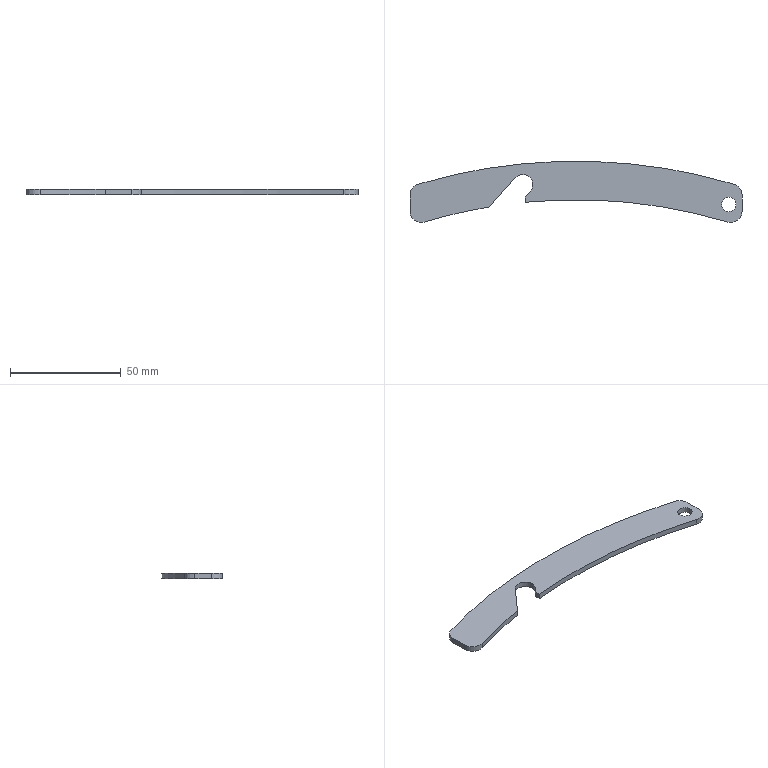Part | SolidWorks | features Fillet 1, FlatPattern 1, ICE 1, SMBaseFlange 1, SheetMetal 1 | 1 solid | 18 faces | box 150 x 27.697 x 2.5 mm | volume 6095 mm3 | cylinder 11 | plane 7 | commonest cylinder face diameters 10 x4 6.5 x2 9 x2 477.484 x2 500 x1
STEP:
#1=CARTESIAN_POINT('',(65.75,-8.,-2.5));
#2=VERTEX_POINT('',#1);
#3=CARTESIAN_POINT('',(72.25,-8.,-2.5));
#4=VERTEX_POINT('',#3);
#5=CARTESIAN_POINT('',(69.,-8.,-2.5));
#6=DIRECTION('',(0.,0.,1.));
#7=DIRECTION('',(1.,0.,0.));
#8=AXIS2_PLACEMENT_3D('',#5,#6,#7);
#9=CIRCLE('',#8,3.25);
#10=EDGE_CURVE('',#2,#4,#9,.T.);
#11=ORIENTED_EDGE('',*,*,#10,.F.);
#12=CARTESIAN_POINT('',(65.75,-8.,0.));
#13=VERTEX_POINT('',#12);
#14=CARTESIAN_POINT('',(65.75,-8.,-2.5));
#15=DIRECTION('',(0.,0.,1.));
#16=VECTOR('',#15,1000.);
#17=LINE('',#14,#16);
#18=EDGE_CURVE('',#2,#13,#17,.T.);
#19=ORIENTED_EDGE('',*,*,#18,.T.);
#20=CARTESIAN_POINT('',(72.25,-8.,0.));
#21=VERTEX_POINT('',#20);
#22=CARTESIAN_POINT('',(69.,-8.,0.));
#23=DIRECTION('',(0.,0.,1.));
#24=DIRECTION('',(1.,0.,0.));
#25=AXIS2_PLACEMENT_3D('',#22,#23,#24);
#26=CIRCLE('',#25,3.25);
#27=EDGE_CURVE('',#13,#21,#26,.T.);
#28=ORIENTED_EDGE('',*,*,#27,.T.);
#29=CARTESIAN_POINT('',(72.25,-8.,-2.5));
#30=DIRECTION('',(0.,0.,1.));
#31=VECTOR('',#30,1000.);
#32=LINE('',#29,#31);
#33=EDGE_CURVE('',#4,#21,#32,.T.);
#34=ORIENTED_EDGE('',*,*,#33,.F.);
#35=EDGE_LOOP('',(#11,#19,#28,#34));
#36=FACE_OUTER_BOUND('',#35,.T.);
#37=CARTESIAN_POINT('',(69.,-8.,-2.5));
#38=DIRECTION('',(0.,0.,1.));
#39=DIRECTION('',(1.,0.,0.));
#40=AXIS2_PLACEMENT_3D('',#37,#38,#39);
#41=CYLINDRICAL_SURFACE('',#40,3.25);
#42=ADVANCED_FACE('',(#36),#41,.F.);
#43=CARTESIAN_POINT('',(-27.362,4.,-2.5));
#44=VERTEX_POINT('',#43);
#45=CARTESIAN_POINT('',(-19.508,1.,-2.5));
#46=VERTEX_POINT('',#45);
#47=CARTESIAN_POINT('',(-24.008,1.,-2.5));
#48=DIRECTION('',(0.,0.,-1.));
#49=DIRECTION('',(-1.,0.,0.));
#50=AXIS2_PLACEMENT_3D('',#47,#48,#49);
#51=CIRCLE('',#50,4.5);
#52=EDGE_CURVE('',#44,#46,#51,.T.);
#53=ORIENTED_EDGE('',*,*,#52,.T.);
#54=CARTESIAN_POINT('',(-19.508,1.,0.));
#55=VERTEX_POINT('',#54);
#56=CARTESIAN_POINT('',(-19.508,1.,-2.5));
#57=DIRECTION('',(0.,0.,1.));
#58=VECTOR('',#57,1000.);
#59=LINE('',#56,#58);
#60=EDGE_CURVE('',#46,#55,#59,.T.);
#61=ORIENTED_EDGE('',*,*,#60,.T.);
#62=CARTESIAN_POINT('',(-27.362,4.,0.));
#63=VERTEX_POINT('',#62);
#64=CARTESIAN_POINT('',(-24.008,1.,0.));
#65=DIRECTION('',(0.,0.,-1.));
#66=DIRECTION('',(-1.,0.,0.));
#67=AXIS2_PLACEMENT_3D('',#64,#65,#66);
#68=CIRCLE('',#67,4.5);
#69=EDGE_CURVE('',#63,#55,#68,.T.);
#70=ORIENTED_EDGE('',*,*,#69,.F.);
#71=CARTESIAN_POINT('',(-27.362,4.,-2.5));
#72=DIRECTION('',(0.,0.,1.));
#73=VECTOR('',#72,1000.);
#74=LINE('',#71,#73);
#75=EDGE_CURVE('',#44,#63,#74,.T.);
#76=ORIENTED_EDGE('',*,*,#75,.F.);
#77=EDGE_LOOP('',(#53,#61,#70,#76));
#78=FACE_OUTER_BOUND('',#77,.T.);
#79=CARTESIAN_POINT('',(-24.008,1.,-2.5));
#80=DIRECTION('',(0.,0.,1.));
#81=DIRECTION('',(1.,0.,0.));
#82=AXIS2_PLACEMENT_3D('',#79,#80,#81);
#83=CYLINDRICAL_SURFACE('',#82,4.5);
#84=ADVANCED_FACE('',(#78),#83,.F.);
#85=CARTESIAN_POINT('',(-23.008,-7.025,0.));
#86=VERTEX_POINT('',#85);
#87=CARTESIAN_POINT('',(68.564,-15.971,0.));
#88=VERTEX_POINT('',#87);
#89=CARTESIAN_POINT('',(0.,-244.656,0.));
#90=DIRECTION('',(0.,0.,-1.));
#91=DIRECTION('',(-1.,0.,0.));
#92=AXIS2_PLACEMENT_3D('',#89,#90,#91);
#93=CIRCLE('',#92,238.742);
#94=EDGE_CURVE('',#86,#88,#93,.T.);
#95=ORIENTED_EDGE('',*,*,#94,.F.);
#96=CARTESIAN_POINT('',(-23.008,-7.025,-2.5));
#97=VERTEX_POINT('',#96);
#98=CARTESIAN_POINT('',(-23.008,-7.025,-2.5));
#99=DIRECTION('',(0.,0.,1.));
#100=VECTOR('',#99,1000.);
#101=LINE('',#98,#100);
#102=EDGE_CURVE('',#97,#86,#101,.T.);
#103=ORIENTED_EDGE('',*,*,#102,.F.);
#104=CARTESIAN_POINT('',(68.564,-15.971,-2.5));
#105=VERTEX_POINT('',#104);
#106=CARTESIAN_POINT('',(0.,-244.656,-2.5));
#107=DIRECTION('',(0.,0.,-1.));
#108=DIRECTION('',(-1.,0.,0.));
#109=AXIS2_PLACEMENT_3D('',#106,#107,#108);
#110=CIRCLE('',#109,238.742);
#111=EDGE_CURVE('',#97,#105,#110,.T.);
#112=ORIENTED_EDGE('',*,*,#111,.T.);
#113=CARTESIAN_POINT('',(68.564,-15.971,-2.5));
#114=DIRECTION('',(0.,0.,1.));
#115=VECTOR('',#114,1000.);
#116=LINE('',#113,#115);
#117=EDGE_CURVE('',#105,#88,#116,.T.);
#118=ORIENTED_EDGE('',*,*,#117,.T.);
#119=EDGE_LOOP('',(#95,#103,#112,#118));
#120=FACE_OUTER_BOUND('',#119,.T.);
#121=CARTESIAN_POINT('',(0.,-244.656,-2.5));
#122=DIRECTION('',(0.,0.,1.));
#123=DIRECTION('',(1.,0.,0.));
#124=AXIS2_PLACEMENT_3D('',#121,#122,#123);
#125=CYLINDRICAL_SURFACE('',#124,238.742);
#126=ADVANCED_FACE('',(#120),#125,.F.);
#127=CARTESIAN_POINT('',(-20.654,-2.,-2.5));
#128=VERTEX_POINT('',#127);
#129=CARTESIAN_POINT('',(-23.008,-4.632,-2.5));
#130=VERTEX_POINT('',#129);
#131=CARTESIAN_POINT('',(-25.363,-7.265,-2.5));
#132=DIRECTION('',(-0.6667,-0.7454,0.));
#133=VECTOR('',#132,1000.);
#134=LINE('',#131,#133);
#135=EDGE_CURVE('',#128,#130,#134,.T.);
#136=ORIENTED_EDGE('',*,*,#135,.T.);
#137=CARTESIAN_POINT('',(-23.008,-4.632,0.));
#138=VERTEX_POINT('',#137);
#139=CARTESIAN_POINT('',(-23.008,-4.632,-2.5));
#140=DIRECTION('',(0.,0.,1.));
#141=VECTOR('',#140,1000.);
#142=LINE('',#139,#141);
#143=EDGE_CURVE('',#130,#138,#142,.T.);
#144=ORIENTED_EDGE('',*,*,#143,.T.);
#145=CARTESIAN_POINT('',(-20.654,-2.,0.));
#146=VERTEX_POINT('',#145);
#147=CARTESIAN_POINT('',(-25.363,-7.265,0.));
#148=DIRECTION('',(-0.6667,-0.7454,0.));
#149=VECTOR('',#148,1000.);
#150=LINE('',#147,#149);
#151=EDGE_CURVE('',#146,#138,#150,.T.);
#152=ORIENTED_EDGE('',*,*,#151,.F.);
#153=CARTESIAN_POINT('',(-20.654,-2.,-2.5));
#154=DIRECTION('',(0.,0.,1.));
#155=VECTOR('',#154,1000.);
#156=LINE('',#153,#155);
#157=EDGE_CURVE('',#128,#146,#156,.T.);
#158=ORIENTED_EDGE('',*,*,#157,.F.);
#159=EDGE_LOOP('',(#136,#144,#152,#158));
#160=FACE_OUTER_BOUND('',#159,.T.);
#161=CARTESIAN_POINT('',(-25.363,-7.265,-2.5));
#162=DIRECTION('',(-0.7454,0.6667,0.));
#163=DIRECTION('',(-0.6667,-0.7454,0.));
#164=AXIS2_PLACEMENT_3D('',#161,#162,#163);
#165=PLANE('',#164);
#166=ADVANCED_FACE('',(#160),#165,.T.);
#167=CARTESIAN_POINT('',(69.,-8.,-2.5));
#168=DIRECTION('',(0.,0.,1.));
#169=DIRECTION('',(1.,0.,0.));
#170=AXIS2_PLACEMENT_3D('',#167,#168,#169);
#171=CIRCLE('',#170,3.25);
#172=EDGE_CURVE('',#4,#2,#171,.T.);
#173=ORIENTED_EDGE('',*,*,#172,.T.);
#174=ORIENTED_EDGE('',*,*,#10,.T.);
#175=EDGE_LOOP('',(#173,#174));
#176=FACE_BOUND('',#175,.T.);
#177=ORIENTED_EDGE('',*,*,#111,.F.);
#178=CARTESIAN_POINT('',(-23.008,-238.485,-2.5));
#179=DIRECTION('',(0.,-1.,0.));
#180=VECTOR('',#179,1000.);
#181=LINE('',#178,#180);
#182=EDGE_CURVE('',#130,#97,#181,.T.);
#183=ORIENTED_EDGE('',*,*,#182,.F.);
#184=ORIENTED_EDGE('',*,*,#135,.F.);
#185=CARTESIAN_POINT('',(-24.008,1.,-2.5));
#186=DIRECTION('',(0.,0.,-1.));
#187=DIRECTION('',(-1.,0.,0.));
#188=AXIS2_PLACEMENT_3D('',#185,#186,#187);
#189=CIRCLE('',#188,4.5);
#190=EDGE_CURVE('',#46,#128,#189,.T.);
#191=ORIENTED_EDGE('',*,*,#190,.F.);
#192=ORIENTED_EDGE('',*,*,#52,.F.);
#193=CARTESIAN_POINT('',(-39.114,-9.139,-2.5));
#194=VERTEX_POINT('',#193);
#195=CARTESIAN_POINT('',(-27.362,4.,-2.5));
#196=DIRECTION('',(0.6667,0.7454,0.));
#197=VECTOR('',#196,1000.);
#198=LINE('',#195,#197);
#199=EDGE_CURVE('',#194,#44,#198,.T.);
#200=ORIENTED_EDGE('',*,*,#199,.F.);
#201=CARTESIAN_POINT('',(-68.564,-15.971,-2.5));
#202=VERTEX_POINT('',#201);
#203=CARTESIAN_POINT('',(0.,-244.656,-2.5));
#204=DIRECTION('',(0.,0.,-1.));
#205=DIRECTION('',(-1.,0.,0.));
#206=AXIS2_PLACEMENT_3D('',#203,#204,#205);
#207=CIRCLE('',#206,238.742);
#208=EDGE_CURVE('',#202,#194,#207,.T.);
#209=ORIENTED_EDGE('',*,*,#208,.F.);
#210=CARTESIAN_POINT('',(-75.,-11.181,-2.5));
#211=VERTEX_POINT('',#210);
#212=CARTESIAN_POINT('',(-70.,-11.181,-2.5));
#213=DIRECTION('',(0.,0.,-1.));
#214=DIRECTION('',(-1.,0.,0.));
#215=AXIS2_PLACEMENT_3D('',#212,#213,#214);
#216=CIRCLE('',#215,5.);
#217=EDGE_CURVE('',#202,#211,#216,.T.);
#218=ORIENTED_EDGE('',*,*,#217,.T.);
#219=CARTESIAN_POINT('',(-75.,-3.698,-2.5));
#220=VERTEX_POINT('',#219);
#221=CARTESIAN_POINT('',(-75.,0.,-2.5));
#222=DIRECTION('',(0.,-1.,0.));
#223=VECTOR('',#222,1000.);
#224=LINE('',#221,#223);
#225=EDGE_CURVE('',#220,#211,#224,.T.);
#226=ORIENTED_EDGE('',*,*,#225,.F.);
#227=CARTESIAN_POINT('',(-71.429,1.094,-2.5));
#228=VERTEX_POINT('',#227);
#229=CARTESIAN_POINT('',(-70.,-3.698,-2.5));
#230=DIRECTION('',(0.,0.,-1.));
#231=DIRECTION('',(-1.,0.,0.));
#232=AXIS2_PLACEMENT_3D('',#229,#230,#231);
#233=CIRCLE('',#232,5.);
#234=EDGE_CURVE('',#220,#228,#233,.T.);
#235=ORIENTED_EDGE('',*,*,#234,.T.);
#236=CARTESIAN_POINT('',(71.429,1.094,-2.5));
#237=VERTEX_POINT('',#236);
#238=CARTESIAN_POINT('',(0.,-238.485,-2.5));
#239=DIRECTION('',(0.,0.,1.));
#240=DIRECTION('',(-1.,0.,0.));
#241=AXIS2_PLACEMENT_3D('',#238,#239,#240);
#242=CIRCLE('',#241,250.);
#243=EDGE_CURVE('',#237,#228,#242,.T.);
#244=ORIENTED_EDGE('',*,*,#243,.F.);
#245=CARTESIAN_POINT('',(75.,-3.698,-2.5));
#246=VERTEX_POINT('',#245);
#247=CARTESIAN_POINT('',(70.,-3.698,-2.5));
#248=DIRECTION('',(0.,0.,-1.));
#249=DIRECTION('',(-1.,0.,0.));
#250=AXIS2_PLACEMENT_3D('',#247,#248,#249);
#251=CIRCLE('',#250,5.);
#252=EDGE_CURVE('',#237,#246,#251,.T.);
#253=ORIENTED_EDGE('',*,*,#252,.T.);
#254=CARTESIAN_POINT('',(75.,-11.181,-2.5));
#255=VERTEX_POINT('',#254);
#256=CARTESIAN_POINT('',(75.,0.,-2.5));
#257=DIRECTION('',(0.,1.,0.));
#258=VECTOR('',#257,1000.);
#259=LINE('',#256,#258);
#260=EDGE_CURVE('',#255,#246,#259,.T.);
#261=ORIENTED_EDGE('',*,*,#260,.F.);
#262=CARTESIAN_POINT('',(70.,-11.181,-2.5));
#263=DIRECTION('',(0.,0.,-1.));
#264=DIRECTION('',(-1.,0.,0.));
#265=AXIS2_PLACEMENT_3D('',#262,#263,#264);
#266=CIRCLE('',#265,5.);
#267=EDGE_CURVE('',#255,#105,#266,.T.);
#268=ORIENTED_EDGE('',*,*,#267,.T.);
#269=EDGE_LOOP('',(#177,#183,#184,#191,#192,#200,#209,#218,#226,#235,#244,#253,#261,#268));
#270=FACE_OUTER_BOUND('',#269,.T.);
#271=CARTESIAN_POINT('',(0.,-238.485,-2.5));
#272=DIRECTION('',(0.,0.,-1.));
#273=DIRECTION('',(-1.,0.,0.));
#274=AXIS2_PLACEMENT_3D('',#271,#272,#273);
#275=PLANE('',#274);
#276=ADVANCED_FACE('',(#176,#270),#275,.T.);
#277=CARTESIAN_POINT('',(69.,-8.,0.));
#278=DIRECTION('',(0.,0.,1.));
#279=DIRECTION('',(1.,0.,0.));
#280=AXIS2_PLACEMENT_3D('',#277,#278,#279);
#281=CIRCLE('',#280,3.25);
#282=EDGE_CURVE('',#21,#13,#281,.T.);
#283=ORIENTED_EDGE('',*,*,#282,.F.);
#284=ORIENTED_EDGE('',*,*,#27,.F.);
#285=EDGE_LOOP('',(#283,#284));
#286=FACE_BOUND('',#285,.T.);
#287=CARTESIAN_POINT('',(-23.008,-238.485,0.));
#288=DIRECTION('',(0.,-1.,0.));
#289=VECTOR('',#288,1000.);
#290=LINE('',#287,#289);
#291=EDGE_CURVE('',#138,#86,#290,.T.);
#292=ORIENTED_EDGE('',*,*,#291,.T.);
#293=ORIENTED_EDGE('',*,*,#94,.T.);
#294=CARTESIAN_POINT('',(75.,-11.181,0.));
#295=VERTEX_POINT('',#294);
#296=CARTESIAN_POINT('',(70.,-11.181,0.));
#297=DIRECTION('',(0.,0.,1.));
#298=DIRECTION('',(-1.,0.,0.));
#299=AXIS2_PLACEMENT_3D('',#296,#297,#298);
#300=CIRCLE('',#299,5.);
#301=EDGE_CURVE('',#88,#295,#300,.T.);
#302=ORIENTED_EDGE('',*,*,#301,.T.);
#303=CARTESIAN_POINT('',(75.,-3.698,0.));
#304=VERTEX_POINT('',#303);
#305=CARTESIAN_POINT('',(75.,0.,0.));
#306=DIRECTION('',(0.,1.,0.));
#307=VECTOR('',#306,1000.);
#308=LINE('',#305,#307);
#309=EDGE_CURVE('',#295,#304,#308,.T.);
#310=ORIENTED_EDGE('',*,*,#309,.T.);
#311=CARTESIAN_POINT('',(71.429,1.094,0.));
#312=VERTEX_POINT('',#311);
#313=CARTESIAN_POINT('',(70.,-3.698,0.));
#314=DIRECTION('',(0.,0.,1.));
#315=DIRECTION('',(-1.,0.,0.));
#316=AXIS2_PLACEMENT_3D('',#313,#314,#315);
#317=CIRCLE('',#316,5.);
#318=EDGE_CURVE('',#304,#312,#317,.T.);
#319=ORIENTED_EDGE('',*,*,#318,.T.);
#320=CARTESIAN_POINT('',(-71.429,1.094,0.));
#321=VERTEX_POINT('',#320);
#322=CARTESIAN_POINT('',(0.,-238.485,0.));
#323=DIRECTION('',(0.,0.,1.));
#324=DIRECTION('',(-1.,0.,0.));
#325=AXIS2_PLACEMENT_3D('',#322,#323,#324);
#326=CIRCLE('',#325,250.);
#327=EDGE_CURVE('',#312,#321,#326,.T.);
#328=ORIENTED_EDGE('',*,*,#327,.T.);
#329=CARTESIAN_POINT('',(-75.,-3.698,0.));
#330=VERTEX_POINT('',#329);
#331=CARTESIAN_POINT('',(-70.,-3.698,0.));
#332=DIRECTION('',(0.,0.,1.));
#333=DIRECTION('',(-1.,0.,0.));
#334=AXIS2_PLACEMENT_3D('',#331,#332,#333);
#335=CIRCLE('',#334,5.);
#336=EDGE_CURVE('',#321,#330,#335,.T.);
#337=ORIENTED_EDGE('',*,*,#336,.T.);
#338=CARTESIAN_POINT('',(-75.,-11.181,0.));
#339=VERTEX_POINT('',#338);
#340=CARTESIAN_POINT('',(-75.,0.,0.));
#341=DIRECTION('',(0.,-1.,0.));
#342=VECTOR('',#341,1000.);
#343=LINE('',#340,#342);
#344=EDGE_CURVE('',#330,#339,#343,.T.);
#345=ORIENTED_EDGE('',*,*,#344,.T.);
#346=CARTESIAN_POINT('',(-68.564,-15.971,0.));
#347=VERTEX_POINT('',#346);
#348=CARTESIAN_POINT('',(-70.,-11.181,0.));
#349=DIRECTION('',(0.,0.,1.));
#350=DIRECTION('',(-1.,0.,0.));
#351=AXIS2_PLACEMENT_3D('',#348,#349,#350);
#352=CIRCLE('',#351,5.);
#353=EDGE_CURVE('',#339,#347,#352,.T.);
#354=ORIENTED_EDGE('',*,*,#353,.T.);
#355=CARTESIAN_POINT('',(-39.114,-9.139,0.));
#356=VERTEX_POINT('',#355);
#357=CARTESIAN_POINT('',(0.,-244.656,0.));
#358=DIRECTION('',(0.,0.,-1.));
#359=DIRECTION('',(-1.,0.,0.));
#360=AXIS2_PLACEMENT_3D('',#357,#358,#359);
#361=CIRCLE('',#360,238.742);
#362=EDGE_CURVE('',#347,#356,#361,.T.);
#363=ORIENTED_EDGE('',*,*,#362,.T.);
#364=CARTESIAN_POINT('',(-27.362,4.,0.));
#365=DIRECTION('',(0.6667,0.7454,0.));
#366=VECTOR('',#365,1000.);
#367=LINE('',#364,#366);
#368=EDGE_CURVE('',#356,#63,#367,.T.);
#369=ORIENTED_EDGE('',*,*,#368,.T.);
#370=ORIENTED_EDGE('',*,*,#69,.T.);
#371=CARTESIAN_POINT('',(-24.008,1.,0.));
#372=DIRECTION('',(0.,0.,-1.));
#373=DIRECTION('',(-1.,0.,0.));
#374=AXIS2_PLACEMENT_3D('',#371,#372,#373);
#375=CIRCLE('',#374,4.5);
#376=EDGE_CURVE('',#55,#146,#375,.T.);
#377=ORIENTED_EDGE('',*,*,#376,.T.);
#378=ORIENTED_EDGE('',*,*,#151,.T.);
#379=EDGE_LOOP('',(#292,#293,#302,#310,#319,#328,#337,#345,#354,#363,#369,#370,#377,#378));
#380=FACE_OUTER_BOUND('',#379,.T.);
#381=CARTESIAN_POINT('',(0.,-238.485,0.));
#382=DIRECTION('',(0.,0.,-1.));
#383=DIRECTION('',(-1.,0.,0.));
#384=AXIS2_PLACEMENT_3D('',#381,#382,#383);
#385=PLANE('',#384);
#386=ADVANCED_FACE('',(#286,#380),#385,.F.);
#387=ORIENTED_EDGE('',*,*,#243,.T.);
#388=CARTESIAN_POINT('',(-71.429,1.094,-2.5));
#389=DIRECTION('',(0.,0.,1.));
#390=VECTOR('',#389,1000.);
#391=LINE('',#388,#390);
#392=EDGE_CURVE('',#228,#321,#391,.T.);
#393=ORIENTED_EDGE('',*,*,#392,.T.);
#394=ORIENTED_EDGE('',*,*,#327,.F.);
#395=CARTESIAN_POINT('',(71.429,1.094,-2.5));
#396=DIRECTION('',(0.,0.,-1.));
#397=VECTOR('',#396,1000.);
#398=LINE('',#395,#397);
#399=EDGE_CURVE('',#312,#237,#398,.T.);
#400=ORIENTED_EDGE('',*,*,#399,.T.);
#401=EDGE_LOOP('',(#387,#393,#394,#400));
#402=FACE_OUTER_BOUND('',#401,.T.);
#403=CARTESIAN_POINT('',(0.,-238.485,-2.5));
#404=DIRECTION('',(0.,0.,1.));
#405=DIRECTION('',(1.,0.,0.));
#406=AXIS2_PLACEMENT_3D('',#403,#404,#405);
#407=CYLINDRICAL_SURFACE('',#406,250.);
#408=ADVANCED_FACE('',(#402),#407,.T.);
#409=ORIENTED_EDGE('',*,*,#309,.F.);
#410=CARTESIAN_POINT('',(75.,-11.181,-2.5));
#411=DIRECTION('',(0.,0.,-1.));
#412=VECTOR('',#411,1000.);
#413=LINE('',#410,#412);
#414=EDGE_CURVE('',#295,#255,#413,.T.);
#415=ORIENTED_EDGE('',*,*,#414,.T.);
#416=ORIENTED_EDGE('',*,*,#260,.T.);
#417=CARTESIAN_POINT('',(75.,-3.698,-2.5));
#418=DIRECTION('',(0.,0.,1.));
#419=VECTOR('',#418,1000.);
#420=LINE('',#417,#419);
#421=EDGE_CURVE('',#246,#304,#420,.T.);
#422=ORIENTED_EDGE('',*,*,#421,.T.);
#423=EDGE_LOOP('',(#409,#415,#416,#422));
#424=FACE_OUTER_BOUND('',#423,.T.);
#425=CARTESIAN_POINT('',(75.,0.,-2.5));
#426=DIRECTION('',(1.,0.,0.));
#427=DIRECTION('',(0.,1.,0.));
#428=AXIS2_PLACEMENT_3D('',#425,#426,#427);
#429=PLANE('',#428);
#430=ADVANCED_FACE('',(#424),#429,.T.);
#431=ORIENTED_EDGE('',*,*,#60,.F.);
#432=ORIENTED_EDGE('',*,*,#190,.T.);
#433=ORIENTED_EDGE('',*,*,#157,.T.);
#434=ORIENTED_EDGE('',*,*,#376,.F.);
#435=EDGE_LOOP('',(#431,#432,#433,#434));
#436=FACE_OUTER_BOUND('',#435,.T.);
#437=CARTESIAN_POINT('',(-24.008,1.,-2.5));
#438=DIRECTION('',(0.,0.,1.));
#439=DIRECTION('',(1.,0.,0.));
#440=AXIS2_PLACEMENT_3D('',#437,#438,#439);
#441=CYLINDRICAL_SURFACE('',#440,4.5);
#442=ADVANCED_FACE('',(#436),#441,.F.);
#443=ORIENTED_EDGE('',*,*,#368,.F.);
#444=CARTESIAN_POINT('',(-39.114,-9.139,-2.5));
#445=DIRECTION('',(0.,0.,1.));
#446=VECTOR('',#445,1000.);
#447=LINE('',#444,#446);
#448=EDGE_CURVE('',#194,#356,#447,.T.);
#449=ORIENTED_EDGE('',*,*,#448,.F.);
#450=ORIENTED_EDGE('',*,*,#199,.T.);
#451=ORIENTED_EDGE('',*,*,#75,.T.);
#452=EDGE_LOOP('',(#443,#449,#450,#451));
#453=FACE_OUTER_BOUND('',#452,.T.);
#454=CARTESIAN_POINT('',(-27.362,4.,-2.5));
#455=DIRECTION('',(0.7454,-0.6667,0.));
#456=DIRECTION('',(0.6667,0.7454,0.));
#457=AXIS2_PLACEMENT_3D('',#454,#455,#456);
#458=PLANE('',#457);
#459=ADVANCED_FACE('',(#453),#458,.T.);
#460=ORIENTED_EDGE('',*,*,#362,.F.);
#461=CARTESIAN_POINT('',(-68.564,-15.971,-2.5));
#462=DIRECTION('',(0.,0.,-1.));
#463=VECTOR('',#462,1000.);
#464=LINE('',#461,#463);
#465=EDGE_CURVE('',#347,#202,#464,.T.);
#466=ORIENTED_EDGE('',*,*,#465,.T.);
#467=ORIENTED_EDGE('',*,*,#208,.T.);
#468=ORIENTED_EDGE('',*,*,#448,.T.);
#469=EDGE_LOOP('',(#460,#466,#467,#468));
#470=FACE_OUTER_BOUND('',#469,.T.);
#471=CARTESIAN_POINT('',(0.,-244.656,-2.5));
#472=DIRECTION('',(0.,0.,1.));
#473=DIRECTION('',(1.,0.,0.));
#474=AXIS2_PLACEMENT_3D('',#471,#472,#473);
#475=CYLINDRICAL_SURFACE('',#474,238.742);
#476=ADVANCED_FACE('',(#470),#475,.F.);
#477=ORIENTED_EDGE('',*,*,#344,.F.);
#478=CARTESIAN_POINT('',(-75.,-3.698,-2.5));
#479=DIRECTION('',(0.,0.,-1.));
#480=VECTOR('',#479,1000.);
#481=LINE('',#478,#480);
#482=EDGE_CURVE('',#330,#220,#481,.T.);
#483=ORIENTED_EDGE('',*,*,#482,.T.);
#484=ORIENTED_EDGE('',*,*,#225,.T.);
#485=CARTESIAN_POINT('',(-75.,-11.181,-2.5));
#486=DIRECTION('',(0.,0.,1.));
#487=VECTOR('',#486,1000.);
#488=LINE('',#485,#487);
#489=EDGE_CURVE('',#211,#339,#488,.T.);
#490=ORIENTED_EDGE('',*,*,#489,.T.);
#491=EDGE_LOOP('',(#477,#483,#484,#490));
#492=FACE_OUTER_BOUND('',#491,.T.);
#493=CARTESIAN_POINT('',(-75.,0.,-2.5));
#494=DIRECTION('',(-1.,0.,0.));
#495=DIRECTION('',(0.,0.,1.));
#496=AXIS2_PLACEMENT_3D('',#493,#494,#495);
#497=PLANE('',#496);
#498=ADVANCED_FACE('',(#492),#497,.T.);
#499=ORIENTED_EDGE('',*,*,#18,.F.);
#500=ORIENTED_EDGE('',*,*,#172,.F.);
#501=ORIENTED_EDGE('',*,*,#33,.T.);
#502=ORIENTED_EDGE('',*,*,#282,.T.);
#503=EDGE_LOOP('',(#499,#500,#501,#502));
#504=FACE_OUTER_BOUND('',#503,.T.);
#505=CARTESIAN_POINT('',(69.,-8.,-2.5));
#506=DIRECTION('',(0.,0.,1.));
#507=DIRECTION('',(1.,0.,0.));
#508=AXIS2_PLACEMENT_3D('',#505,#506,#507);
#509=CYLINDRICAL_SURFACE('',#508,3.25);
#510=ADVANCED_FACE('',(#504),#509,.F.);
#511=ORIENTED_EDGE('',*,*,#234,.F.);
#512=ORIENTED_EDGE('',*,*,#482,.F.);
#513=ORIENTED_EDGE('',*,*,#336,.F.);
#514=ORIENTED_EDGE('',*,*,#392,.F.);
#515=EDGE_LOOP('',(#511,#512,#513,#514));
#516=FACE_OUTER_BOUND('',#515,.T.);
#517=CARTESIAN_POINT('',(-70.,-3.698,-2.5));
#518=DIRECTION('',(0.,0.,1.));
#519=DIRECTION('',(1.,0.,0.));
#520=AXIS2_PLACEMENT_3D('',#517,#518,#519);
#521=CYLINDRICAL_SURFACE('',#520,5.);
#522=ADVANCED_FACE('',(#516),#521,.T.);
#523=ORIENTED_EDGE('',*,*,#217,.F.);
#524=ORIENTED_EDGE('',*,*,#465,.F.);
#525=ORIENTED_EDGE('',*,*,#353,.F.);
#526=ORIENTED_EDGE('',*,*,#489,.F.);
#527=EDGE_LOOP('',(#523,#524,#525,#526));
#528=FACE_OUTER_BOUND('',#527,.T.);
#529=CARTESIAN_POINT('',(-70.,-11.181,-2.5));
#530=DIRECTION('',(0.,0.,1.));
#531=DIRECTION('',(1.,0.,0.));
#532=AXIS2_PLACEMENT_3D('',#529,#530,#531);
#533=CYLINDRICAL_SURFACE('',#532,5.);
#534=ADVANCED_FACE('',(#528),#533,.T.);
#535=ORIENTED_EDGE('',*,*,#267,.F.);
#536=ORIENTED_EDGE('',*,*,#414,.F.);
#537=ORIENTED_EDGE('',*,*,#301,.F.);
#538=ORIENTED_EDGE('',*,*,#117,.F.);
#539=EDGE_LOOP('',(#535,#536,#537,#538));
#540=FACE_OUTER_BOUND('',#539,.T.);
#541=CARTESIAN_POINT('',(70.,-11.181,-2.5));
#542=DIRECTION('',(0.,0.,1.));
#543=DIRECTION('',(1.,0.,0.));
#544=AXIS2_PLACEMENT_3D('',#541,#542,#543);
#545=CYLINDRICAL_SURFACE('',#544,5.);
#546=ADVANCED_FACE('',(#540),#545,.T.);
#547=ORIENTED_EDGE('',*,*,#252,.F.);
#548=ORIENTED_EDGE('',*,*,#399,.F.);
#549=ORIENTED_EDGE('',*,*,#318,.F.);
#550=ORIENTED_EDGE('',*,*,#421,.F.);
#551=EDGE_LOOP('',(#547,#548,#549,#550));
#552=FACE_OUTER_BOUND('',#551,.T.);
#553=CARTESIAN_POINT('',(70.,-3.698,-2.5));
#554=DIRECTION('',(0.,0.,1.));
#555=DIRECTION('',(1.,0.,0.));
#556=AXIS2_PLACEMENT_3D('',#553,#554,#555);
#557=CYLINDRICAL_SURFACE('',#556,5.);
#558=ADVANCED_FACE('',(#552),#557,.T.);
#559=ORIENTED_EDGE('',*,*,#182,.T.);
#560=ORIENTED_EDGE('',*,*,#102,.T.);
#561=ORIENTED_EDGE('',*,*,#291,.F.);
#562=ORIENTED_EDGE('',*,*,#143,.F.);
#563=EDGE_LOOP('',(#559,#560,#561,#562));
#564=FACE_OUTER_BOUND('',#563,.T.);
#565=CARTESIAN_POINT('',(-23.008,-238.485,-2.5));
#566=DIRECTION('',(1.,0.,0.));
#567=DIRECTION('',(0.,-1.,0.));
#568=AXIS2_PLACEMENT_3D('',#565,#566,#567);
#569=PLANE('',#568);
#570=ADVANCED_FACE('',(#564),#569,.F.);
#571=CLOSED_SHELL('',(#42,#84,#126,#166,#276,#386,#408,#430,#442,#459,#476,#498,#510,#522,#534,#546,#558,#570));
#572=MANIFOLD_SOLID_BREP('',#571);
#573=CARTESIAN_POINT('',(0.,0.,0.));
#574=DIRECTION('',(0.,0.,1.));
#575=DIRECTION('',(1.,0.,0.));
#576=AXIS2_PLACEMENT_3D('',#573,#574,#575);
#577=(LENGTH_UNIT()NAMED_UNIT(*)SI_UNIT(.MILLI.,.METRE.));
#578=UNCERTAINTY_MEASURE_WITH_UNIT(LENGTH_MEASURE(0.00001),#577,'','');
#579=(NAMED_UNIT(*)PLANE_ANGLE_UNIT()SI_UNIT($,.RADIAN.));
#580=(NAMED_UNIT(*)SI_UNIT($,.STERADIAN.)SOLID_ANGLE_UNIT());
#581=(GEOMETRIC_REPRESENTATION_CONTEXT(3)GLOBAL_UNCERTAINTY_ASSIGNED_CONTEXT((#578))GLOBAL_UNIT_ASSIGNED_CONTEXT((#577,#579,#580))REPRESENTATION_CONTEXT('',''));
#582=ADVANCED_BREP_SHAPE_REPRESENTATION('',(#572,#576),#581);